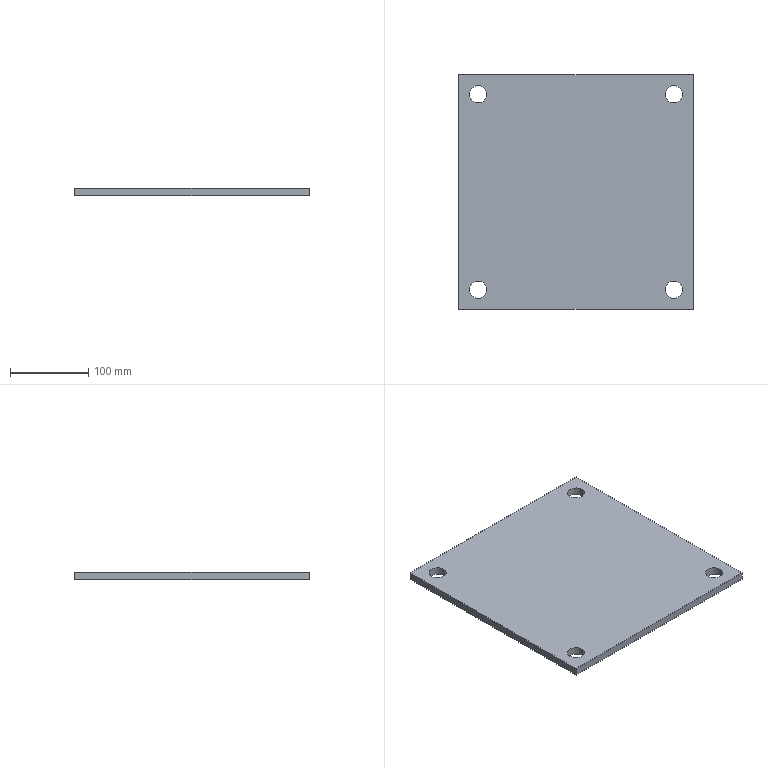Part | SolidWorks | features Extrusion 1 | 1 solid | 14 faces | box 300 x 300 x 10 mm | volume 884795 mm3 | cylinder 8 | plane 6 | commonest cylinder face diameters 22 x8
STEP:
#1=CARTESIAN_POINT('',(-136.,-125.,10.));
#2=VERTEX_POINT('',#1);
#3=CARTESIAN_POINT('',(-114.,-125.,10.));
#4=VERTEX_POINT('',#3);
#5=CARTESIAN_POINT('',(-125.,-125.,10.));
#6=DIRECTION('',(0.,0.,1.));
#7=DIRECTION('',(1.,0.,0.));
#8=AXIS2_PLACEMENT_3D('',#5,#6,#7);
#9=CIRCLE('',#8,11.);
#10=EDGE_CURVE('',#2,#4,#9,.T.);
#11=ORIENTED_EDGE('',*,*,#10,.T.);
#12=CARTESIAN_POINT('',(-114.,-125.,0.));
#13=VERTEX_POINT('',#12);
#14=CARTESIAN_POINT('',(-114.,-125.,10.));
#15=DIRECTION('',(0.,0.,-1.));
#16=VECTOR('',#15,1000.);
#17=LINE('',#14,#16);
#18=EDGE_CURVE('',#4,#13,#17,.T.);
#19=ORIENTED_EDGE('',*,*,#18,.T.);
#20=CARTESIAN_POINT('',(-136.,-125.,0.));
#21=VERTEX_POINT('',#20);
#22=CARTESIAN_POINT('',(-125.,-125.,0.));
#23=DIRECTION('',(0.,0.,1.));
#24=DIRECTION('',(1.,0.,0.));
#25=AXIS2_PLACEMENT_3D('',#22,#23,#24);
#26=CIRCLE('',#25,11.);
#27=EDGE_CURVE('',#21,#13,#26,.T.);
#28=ORIENTED_EDGE('',*,*,#27,.F.);
#29=CARTESIAN_POINT('',(-136.,-125.,10.));
#30=DIRECTION('',(0.,0.,-1.));
#31=VECTOR('',#30,1000.);
#32=LINE('',#29,#31);
#33=EDGE_CURVE('',#2,#21,#32,.T.);
#34=ORIENTED_EDGE('',*,*,#33,.F.);
#35=EDGE_LOOP('',(#11,#19,#28,#34));
#36=FACE_OUTER_BOUND('',#35,.T.);
#37=CARTESIAN_POINT('',(-125.,-125.,10.));
#38=DIRECTION('',(0.,0.,-1.));
#39=DIRECTION('',(-1.,0.,0.));
#40=AXIS2_PLACEMENT_3D('',#37,#38,#39);
#41=CYLINDRICAL_SURFACE('',#40,11.);
#42=ADVANCED_FACE('',(#36),#41,.F.);
#43=CARTESIAN_POINT('',(114.,-125.,10.));
#44=VERTEX_POINT('',#43);
#45=CARTESIAN_POINT('',(136.,-125.,10.));
#46=VERTEX_POINT('',#45);
#47=CARTESIAN_POINT('',(125.,-125.,10.));
#48=DIRECTION('',(0.,0.,1.));
#49=DIRECTION('',(1.,0.,0.));
#50=AXIS2_PLACEMENT_3D('',#47,#48,#49);
#51=CIRCLE('',#50,11.);
#52=EDGE_CURVE('',#44,#46,#51,.T.);
#53=ORIENTED_EDGE('',*,*,#52,.T.);
#54=CARTESIAN_POINT('',(136.,-125.,0.));
#55=VERTEX_POINT('',#54);
#56=CARTESIAN_POINT('',(136.,-125.,10.));
#57=DIRECTION('',(0.,0.,-1.));
#58=VECTOR('',#57,1000.);
#59=LINE('',#56,#58);
#60=EDGE_CURVE('',#46,#55,#59,.T.);
#61=ORIENTED_EDGE('',*,*,#60,.T.);
#62=CARTESIAN_POINT('',(114.,-125.,0.));
#63=VERTEX_POINT('',#62);
#64=CARTESIAN_POINT('',(125.,-125.,0.));
#65=DIRECTION('',(0.,0.,1.));
#66=DIRECTION('',(1.,0.,0.));
#67=AXIS2_PLACEMENT_3D('',#64,#65,#66);
#68=CIRCLE('',#67,11.);
#69=EDGE_CURVE('',#63,#55,#68,.T.);
#70=ORIENTED_EDGE('',*,*,#69,.F.);
#71=CARTESIAN_POINT('',(114.,-125.,10.));
#72=DIRECTION('',(0.,0.,-1.));
#73=VECTOR('',#72,1000.);
#74=LINE('',#71,#73);
#75=EDGE_CURVE('',#44,#63,#74,.T.);
#76=ORIENTED_EDGE('',*,*,#75,.F.);
#77=EDGE_LOOP('',(#53,#61,#70,#76));
#78=FACE_OUTER_BOUND('',#77,.T.);
#79=CARTESIAN_POINT('',(125.,-125.,10.));
#80=DIRECTION('',(0.,0.,-1.));
#81=DIRECTION('',(-1.,0.,0.));
#82=AXIS2_PLACEMENT_3D('',#79,#80,#81);
#83=CYLINDRICAL_SURFACE('',#82,11.);
#84=ADVANCED_FACE('',(#78),#83,.F.);
#85=CARTESIAN_POINT('',(114.,125.,10.));
#86=VERTEX_POINT('',#85);
#87=CARTESIAN_POINT('',(136.,125.,10.));
#88=VERTEX_POINT('',#87);
#89=CARTESIAN_POINT('',(125.,125.,10.));
#90=DIRECTION('',(0.,0.,1.));
#91=DIRECTION('',(1.,0.,0.));
#92=AXIS2_PLACEMENT_3D('',#89,#90,#91);
#93=CIRCLE('',#92,11.);
#94=EDGE_CURVE('',#86,#88,#93,.T.);
#95=ORIENTED_EDGE('',*,*,#94,.T.);
#96=CARTESIAN_POINT('',(136.,125.,0.));
#97=VERTEX_POINT('',#96);
#98=CARTESIAN_POINT('',(136.,125.,10.));
#99=DIRECTION('',(0.,0.,-1.));
#100=VECTOR('',#99,1000.);
#101=LINE('',#98,#100);
#102=EDGE_CURVE('',#88,#97,#101,.T.);
#103=ORIENTED_EDGE('',*,*,#102,.T.);
#104=CARTESIAN_POINT('',(114.,125.,0.));
#105=VERTEX_POINT('',#104);
#106=CARTESIAN_POINT('',(125.,125.,0.));
#107=DIRECTION('',(0.,0.,1.));
#108=DIRECTION('',(1.,0.,0.));
#109=AXIS2_PLACEMENT_3D('',#106,#107,#108);
#110=CIRCLE('',#109,11.);
#111=EDGE_CURVE('',#105,#97,#110,.T.);
#112=ORIENTED_EDGE('',*,*,#111,.F.);
#113=CARTESIAN_POINT('',(114.,125.,10.));
#114=DIRECTION('',(0.,0.,-1.));
#115=VECTOR('',#114,1000.);
#116=LINE('',#113,#115);
#117=EDGE_CURVE('',#86,#105,#116,.T.);
#118=ORIENTED_EDGE('',*,*,#117,.F.);
#119=EDGE_LOOP('',(#95,#103,#112,#118));
#120=FACE_OUTER_BOUND('',#119,.T.);
#121=CARTESIAN_POINT('',(125.,125.,10.));
#122=DIRECTION('',(0.,0.,-1.));
#123=DIRECTION('',(-1.,0.,0.));
#124=AXIS2_PLACEMENT_3D('',#121,#122,#123);
#125=CYLINDRICAL_SURFACE('',#124,11.);
#126=ADVANCED_FACE('',(#120),#125,.F.);
#127=CARTESIAN_POINT('',(-136.,125.,10.));
#128=VERTEX_POINT('',#127);
#129=CARTESIAN_POINT('',(-114.,125.,10.));
#130=VERTEX_POINT('',#129);
#131=CARTESIAN_POINT('',(-125.,125.,10.));
#132=DIRECTION('',(0.,0.,1.));
#133=DIRECTION('',(1.,0.,0.));
#134=AXIS2_PLACEMENT_3D('',#131,#132,#133);
#135=CIRCLE('',#134,11.);
#136=EDGE_CURVE('',#128,#130,#135,.T.);
#137=ORIENTED_EDGE('',*,*,#136,.T.);
#138=CARTESIAN_POINT('',(-114.,125.,0.));
#139=VERTEX_POINT('',#138);
#140=CARTESIAN_POINT('',(-114.,125.,10.));
#141=DIRECTION('',(0.,0.,-1.));
#142=VECTOR('',#141,1000.);
#143=LINE('',#140,#142);
#144=EDGE_CURVE('',#130,#139,#143,.T.);
#145=ORIENTED_EDGE('',*,*,#144,.T.);
#146=CARTESIAN_POINT('',(-136.,125.,0.));
#147=VERTEX_POINT('',#146);
#148=CARTESIAN_POINT('',(-125.,125.,0.));
#149=DIRECTION('',(0.,0.,1.));
#150=DIRECTION('',(1.,0.,0.));
#151=AXIS2_PLACEMENT_3D('',#148,#149,#150);
#152=CIRCLE('',#151,11.);
#153=EDGE_CURVE('',#147,#139,#152,.T.);
#154=ORIENTED_EDGE('',*,*,#153,.F.);
#155=CARTESIAN_POINT('',(-136.,125.,10.));
#156=DIRECTION('',(0.,0.,-1.));
#157=VECTOR('',#156,1000.);
#158=LINE('',#155,#157);
#159=EDGE_CURVE('',#128,#147,#158,.T.);
#160=ORIENTED_EDGE('',*,*,#159,.F.);
#161=EDGE_LOOP('',(#137,#145,#154,#160));
#162=FACE_OUTER_BOUND('',#161,.T.);
#163=CARTESIAN_POINT('',(-125.,125.,10.));
#164=DIRECTION('',(0.,0.,-1.));
#165=DIRECTION('',(-1.,0.,0.));
#166=AXIS2_PLACEMENT_3D('',#163,#164,#165);
#167=CYLINDRICAL_SURFACE('',#166,11.);
#168=ADVANCED_FACE('',(#162),#167,.F.);
#169=ORIENTED_EDGE('',*,*,#52,.F.);
#170=CARTESIAN_POINT('',(125.,-125.,10.));
#171=DIRECTION('',(0.,0.,1.));
#172=DIRECTION('',(1.,0.,0.));
#173=AXIS2_PLACEMENT_3D('',#170,#171,#172);
#174=CIRCLE('',#173,11.);
#175=EDGE_CURVE('',#46,#44,#174,.T.);
#176=ORIENTED_EDGE('',*,*,#175,.F.);
#177=EDGE_LOOP('',(#169,#176));
#178=FACE_BOUND('',#177,.T.);
#179=ORIENTED_EDGE('',*,*,#136,.F.);
#180=CARTESIAN_POINT('',(-125.,125.,10.));
#181=DIRECTION('',(0.,0.,1.));
#182=DIRECTION('',(1.,0.,0.));
#183=AXIS2_PLACEMENT_3D('',#180,#181,#182);
#184=CIRCLE('',#183,11.);
#185=EDGE_CURVE('',#130,#128,#184,.T.);
#186=ORIENTED_EDGE('',*,*,#185,.F.);
#187=EDGE_LOOP('',(#179,#186));
#188=FACE_BOUND('',#187,.T.);
#189=CARTESIAN_POINT('',(150.,-150.,10.));
#190=VERTEX_POINT('',#189);
#191=CARTESIAN_POINT('',(150.,150.,10.));
#192=VERTEX_POINT('',#191);
#193=CARTESIAN_POINT('',(150.,150.,10.));
#194=DIRECTION('',(0.,1.,0.));
#195=VECTOR('',#194,1000.);
#196=LINE('',#193,#195);
#197=EDGE_CURVE('',#190,#192,#196,.T.);
#198=ORIENTED_EDGE('',*,*,#197,.T.);
#199=CARTESIAN_POINT('',(-150.,150.,10.));
#200=VERTEX_POINT('',#199);
#201=CARTESIAN_POINT('',(-150.,150.,10.));
#202=DIRECTION('',(-1.,0.,0.));
#203=VECTOR('',#202,1000.);
#204=LINE('',#201,#203);
#205=EDGE_CURVE('',#192,#200,#204,.T.);
#206=ORIENTED_EDGE('',*,*,#205,.T.);
#207=CARTESIAN_POINT('',(-150.,-150.,10.));
#208=VERTEX_POINT('',#207);
#209=CARTESIAN_POINT('',(-150.,150.,10.));
#210=DIRECTION('',(0.,-1.,0.));
#211=VECTOR('',#210,1000.);
#212=LINE('',#209,#211);
#213=EDGE_CURVE('',#200,#208,#212,.T.);
#214=ORIENTED_EDGE('',*,*,#213,.T.);
#215=CARTESIAN_POINT('',(-150.,-150.,10.));
#216=DIRECTION('',(1.,0.,0.));
#217=VECTOR('',#216,1000.);
#218=LINE('',#215,#217);
#219=EDGE_CURVE('',#208,#190,#218,.T.);
#220=ORIENTED_EDGE('',*,*,#219,.T.);
#221=EDGE_LOOP('',(#198,#206,#214,#220));
#222=FACE_OUTER_BOUND('',#221,.T.);
#223=ORIENTED_EDGE('',*,*,#94,.F.);
#224=CARTESIAN_POINT('',(125.,125.,10.));
#225=DIRECTION('',(0.,0.,1.));
#226=DIRECTION('',(1.,0.,0.));
#227=AXIS2_PLACEMENT_3D('',#224,#225,#226);
#228=CIRCLE('',#227,11.);
#229=EDGE_CURVE('',#88,#86,#228,.T.);
#230=ORIENTED_EDGE('',*,*,#229,.F.);
#231=EDGE_LOOP('',(#223,#230));
#232=FACE_BOUND('',#231,.T.);
#233=ORIENTED_EDGE('',*,*,#10,.F.);
#234=CARTESIAN_POINT('',(-125.,-125.,10.));
#235=DIRECTION('',(0.,0.,1.));
#236=DIRECTION('',(1.,0.,0.));
#237=AXIS2_PLACEMENT_3D('',#234,#235,#236);
#238=CIRCLE('',#237,11.);
#239=EDGE_CURVE('',#4,#2,#238,.T.);
#240=ORIENTED_EDGE('',*,*,#239,.F.);
#241=EDGE_LOOP('',(#233,#240));
#242=FACE_BOUND('',#241,.T.);
#243=CARTESIAN_POINT('',(0.,0.,10.));
#244=DIRECTION('',(0.,0.,1.));
#245=DIRECTION('',(1.,0.,0.));
#246=AXIS2_PLACEMENT_3D('',#243,#244,#245);
#247=PLANE('',#246);
#248=ADVANCED_FACE('',(#178,#188,#222,#232,#242),#247,.T.);
#249=CARTESIAN_POINT('',(150.,-150.,0.));
#250=VERTEX_POINT('',#249);
#251=CARTESIAN_POINT('',(150.,150.,0.));
#252=VERTEX_POINT('',#251);
#253=CARTESIAN_POINT('',(150.,150.,0.));
#254=DIRECTION('',(0.,1.,0.));
#255=VECTOR('',#254,1000.);
#256=LINE('',#253,#255);
#257=EDGE_CURVE('',#250,#252,#256,.T.);
#258=ORIENTED_EDGE('',*,*,#257,.F.);
#259=CARTESIAN_POINT('',(-150.,-150.,0.));
#260=VERTEX_POINT('',#259);
#261=CARTESIAN_POINT('',(-150.,-150.,0.));
#262=DIRECTION('',(1.,0.,0.));
#263=VECTOR('',#262,1000.);
#264=LINE('',#261,#263);
#265=EDGE_CURVE('',#260,#250,#264,.T.);
#266=ORIENTED_EDGE('',*,*,#265,.F.);
#267=CARTESIAN_POINT('',(-150.,150.,0.));
#268=VERTEX_POINT('',#267);
#269=CARTESIAN_POINT('',(-150.,150.,0.));
#270=DIRECTION('',(0.,-1.,0.));
#271=VECTOR('',#270,1000.);
#272=LINE('',#269,#271);
#273=EDGE_CURVE('',#268,#260,#272,.T.);
#274=ORIENTED_EDGE('',*,*,#273,.F.);
#275=CARTESIAN_POINT('',(-150.,150.,0.));
#276=DIRECTION('',(-1.,0.,0.));
#277=VECTOR('',#276,1000.);
#278=LINE('',#275,#277);
#279=EDGE_CURVE('',#252,#268,#278,.T.);
#280=ORIENTED_EDGE('',*,*,#279,.F.);
#281=EDGE_LOOP('',(#258,#266,#274,#280));
#282=FACE_OUTER_BOUND('',#281,.T.);
#283=ORIENTED_EDGE('',*,*,#153,.T.);
#284=CARTESIAN_POINT('',(-125.,125.,0.));
#285=DIRECTION('',(0.,0.,1.));
#286=DIRECTION('',(1.,0.,0.));
#287=AXIS2_PLACEMENT_3D('',#284,#285,#286);
#288=CIRCLE('',#287,11.);
#289=EDGE_CURVE('',#139,#147,#288,.T.);
#290=ORIENTED_EDGE('',*,*,#289,.T.);
#291=EDGE_LOOP('',(#283,#290));
#292=FACE_BOUND('',#291,.T.);
#293=ORIENTED_EDGE('',*,*,#111,.T.);
#294=CARTESIAN_POINT('',(125.,125.,0.));
#295=DIRECTION('',(0.,0.,1.));
#296=DIRECTION('',(1.,0.,0.));
#297=AXIS2_PLACEMENT_3D('',#294,#295,#296);
#298=CIRCLE('',#297,11.);
#299=EDGE_CURVE('',#97,#105,#298,.T.);
#300=ORIENTED_EDGE('',*,*,#299,.T.);
#301=EDGE_LOOP('',(#293,#300));
#302=FACE_BOUND('',#301,.T.);
#303=ORIENTED_EDGE('',*,*,#69,.T.);
#304=CARTESIAN_POINT('',(125.,-125.,0.));
#305=DIRECTION('',(0.,0.,1.));
#306=DIRECTION('',(1.,0.,0.));
#307=AXIS2_PLACEMENT_3D('',#304,#305,#306);
#308=CIRCLE('',#307,11.);
#309=EDGE_CURVE('',#55,#63,#308,.T.);
#310=ORIENTED_EDGE('',*,*,#309,.T.);
#311=EDGE_LOOP('',(#303,#310));
#312=FACE_BOUND('',#311,.T.);
#313=ORIENTED_EDGE('',*,*,#27,.T.);
#314=CARTESIAN_POINT('',(-125.,-125.,0.));
#315=DIRECTION('',(0.,0.,1.));
#316=DIRECTION('',(1.,0.,0.));
#317=AXIS2_PLACEMENT_3D('',#314,#315,#316);
#318=CIRCLE('',#317,11.);
#319=EDGE_CURVE('',#13,#21,#318,.T.);
#320=ORIENTED_EDGE('',*,*,#319,.T.);
#321=EDGE_LOOP('',(#313,#320));
#322=FACE_BOUND('',#321,.T.);
#323=CARTESIAN_POINT('',(0.,0.,0.));
#324=DIRECTION('',(0.,0.,1.));
#325=DIRECTION('',(1.,0.,0.));
#326=AXIS2_PLACEMENT_3D('',#323,#324,#325);
#327=PLANE('',#326);
#328=ADVANCED_FACE('',(#282,#292,#302,#312,#322),#327,.F.);
#329=ORIENTED_EDGE('',*,*,#257,.T.);
#330=CARTESIAN_POINT('',(150.,150.,10.));
#331=DIRECTION('',(0.,0.,-1.));
#332=VECTOR('',#331,1000.);
#333=LINE('',#330,#332);
#334=EDGE_CURVE('',#192,#252,#333,.T.);
#335=ORIENTED_EDGE('',*,*,#334,.F.);
#336=ORIENTED_EDGE('',*,*,#197,.F.);
#337=CARTESIAN_POINT('',(150.,-150.,10.));
#338=DIRECTION('',(0.,0.,-1.));
#339=VECTOR('',#338,1000.);
#340=LINE('',#337,#339);
#341=EDGE_CURVE('',#190,#250,#340,.T.);
#342=ORIENTED_EDGE('',*,*,#341,.T.);
#343=EDGE_LOOP('',(#329,#335,#336,#342));
#344=FACE_OUTER_BOUND('',#343,.T.);
#345=CARTESIAN_POINT('',(150.,150.,10.));
#346=DIRECTION('',(-1.,0.,0.));
#347=DIRECTION('',(0.,-1.,0.));
#348=AXIS2_PLACEMENT_3D('',#345,#346,#347);
#349=PLANE('',#348);
#350=ADVANCED_FACE('',(#344),#349,.F.);
#351=ORIENTED_EDGE('',*,*,#279,.T.);
#352=CARTESIAN_POINT('',(-150.,150.,10.));
#353=DIRECTION('',(0.,0.,-1.));
#354=VECTOR('',#353,1000.);
#355=LINE('',#352,#354);
#356=EDGE_CURVE('',#200,#268,#355,.T.);
#357=ORIENTED_EDGE('',*,*,#356,.F.);
#358=ORIENTED_EDGE('',*,*,#205,.F.);
#359=ORIENTED_EDGE('',*,*,#334,.T.);
#360=EDGE_LOOP('',(#351,#357,#358,#359));
#361=FACE_OUTER_BOUND('',#360,.T.);
#362=CARTESIAN_POINT('',(-150.,150.,10.));
#363=DIRECTION('',(0.,-1.,0.));
#364=DIRECTION('',(0.,0.,-1.));
#365=AXIS2_PLACEMENT_3D('',#362,#363,#364);
#366=PLANE('',#365);
#367=ADVANCED_FACE('',(#361),#366,.F.);
#368=ORIENTED_EDGE('',*,*,#273,.T.);
#369=CARTESIAN_POINT('',(-150.,-150.,10.));
#370=DIRECTION('',(0.,0.,-1.));
#371=VECTOR('',#370,1000.);
#372=LINE('',#369,#371);
#373=EDGE_CURVE('',#208,#260,#372,.T.);
#374=ORIENTED_EDGE('',*,*,#373,.F.);
#375=ORIENTED_EDGE('',*,*,#213,.F.);
#376=ORIENTED_EDGE('',*,*,#356,.T.);
#377=EDGE_LOOP('',(#368,#374,#375,#376));
#378=FACE_OUTER_BOUND('',#377,.T.);
#379=CARTESIAN_POINT('',(-150.,150.,10.));
#380=DIRECTION('',(1.,0.,0.));
#381=DIRECTION('',(0.,1.,0.));
#382=AXIS2_PLACEMENT_3D('',#379,#380,#381);
#383=PLANE('',#382);
#384=ADVANCED_FACE('',(#378),#383,.F.);
#385=ORIENTED_EDGE('',*,*,#265,.T.);
#386=ORIENTED_EDGE('',*,*,#341,.F.);
#387=ORIENTED_EDGE('',*,*,#219,.F.);
#388=ORIENTED_EDGE('',*,*,#373,.T.);
#389=EDGE_LOOP('',(#385,#386,#387,#388));
#390=FACE_OUTER_BOUND('',#389,.T.);
#391=CARTESIAN_POINT('',(-150.,-150.,10.));
#392=DIRECTION('',(0.,1.,0.));
#393=DIRECTION('',(0.,0.,1.));
#394=AXIS2_PLACEMENT_3D('',#391,#392,#393);
#395=PLANE('',#394);
#396=ADVANCED_FACE('',(#390),#395,.F.);
#397=ORIENTED_EDGE('',*,*,#144,.F.);
#398=ORIENTED_EDGE('',*,*,#185,.T.);
#399=ORIENTED_EDGE('',*,*,#159,.T.);
#400=ORIENTED_EDGE('',*,*,#289,.F.);
#401=EDGE_LOOP('',(#397,#398,#399,#400));
#402=FACE_OUTER_BOUND('',#401,.T.);
#403=CARTESIAN_POINT('',(-125.,125.,10.));
#404=DIRECTION('',(0.,0.,-1.));
#405=DIRECTION('',(-1.,0.,0.));
#406=AXIS2_PLACEMENT_3D('',#403,#404,#405);
#407=CYLINDRICAL_SURFACE('',#406,11.);
#408=ADVANCED_FACE('',(#402),#407,.F.);
#409=ORIENTED_EDGE('',*,*,#102,.F.);
#410=ORIENTED_EDGE('',*,*,#229,.T.);
#411=ORIENTED_EDGE('',*,*,#117,.T.);
#412=ORIENTED_EDGE('',*,*,#299,.F.);
#413=EDGE_LOOP('',(#409,#410,#411,#412));
#414=FACE_OUTER_BOUND('',#413,.T.);
#415=CARTESIAN_POINT('',(125.,125.,10.));
#416=DIRECTION('',(0.,0.,-1.));
#417=DIRECTION('',(-1.,0.,0.));
#418=AXIS2_PLACEMENT_3D('',#415,#416,#417);
#419=CYLINDRICAL_SURFACE('',#418,11.);
#420=ADVANCED_FACE('',(#414),#419,.F.);
#421=ORIENTED_EDGE('',*,*,#60,.F.);
#422=ORIENTED_EDGE('',*,*,#175,.T.);
#423=ORIENTED_EDGE('',*,*,#75,.T.);
#424=ORIENTED_EDGE('',*,*,#309,.F.);
#425=EDGE_LOOP('',(#421,#422,#423,#424));
#426=FACE_OUTER_BOUND('',#425,.T.);
#427=CARTESIAN_POINT('',(125.,-125.,10.));
#428=DIRECTION('',(0.,0.,-1.));
#429=DIRECTION('',(-1.,0.,0.));
#430=AXIS2_PLACEMENT_3D('',#427,#428,#429);
#431=CYLINDRICAL_SURFACE('',#430,11.);
#432=ADVANCED_FACE('',(#426),#431,.F.);
#433=ORIENTED_EDGE('',*,*,#18,.F.);
#434=ORIENTED_EDGE('',*,*,#239,.T.);
#435=ORIENTED_EDGE('',*,*,#33,.T.);
#436=ORIENTED_EDGE('',*,*,#319,.F.);
#437=EDGE_LOOP('',(#433,#434,#435,#436));
#438=FACE_OUTER_BOUND('',#437,.T.);
#439=CARTESIAN_POINT('',(-125.,-125.,10.));
#440=DIRECTION('',(0.,0.,-1.));
#441=DIRECTION('',(-1.,0.,0.));
#442=AXIS2_PLACEMENT_3D('',#439,#440,#441);
#443=CYLINDRICAL_SURFACE('',#442,11.);
#444=ADVANCED_FACE('',(#438),#443,.F.);
#445=CLOSED_SHELL('',(#42,#84,#126,#168,#248,#328,#350,#367,#384,#396,#408,#420,#432,#444));
#446=MANIFOLD_SOLID_BREP('',#445);
#447=CARTESIAN_POINT('',(0.,0.,0.));
#448=DIRECTION('',(0.,0.,1.));
#449=DIRECTION('',(1.,0.,0.));
#450=AXIS2_PLACEMENT_3D('',#447,#448,#449);
#451=(LENGTH_UNIT()NAMED_UNIT(*)SI_UNIT(.MILLI.,.METRE.));
#452=UNCERTAINTY_MEASURE_WITH_UNIT(LENGTH_MEASURE(0.00001),#451,'','');
#453=(NAMED_UNIT(*)PLANE_ANGLE_UNIT()SI_UNIT($,.RADIAN.));
#454=(NAMED_UNIT(*)SI_UNIT($,.STERADIAN.)SOLID_ANGLE_UNIT());
#455=(GEOMETRIC_REPRESENTATION_CONTEXT(3)GLOBAL_UNCERTAINTY_ASSIGNED_CONTEXT((#452))GLOBAL_UNIT_ASSIGNED_CONTEXT((#451,#453,#454))REPRESENTATION_CONTEXT('',''));
#456=ADVANCED_BREP_SHAPE_REPRESENTATION('',(#446,#450),#455);